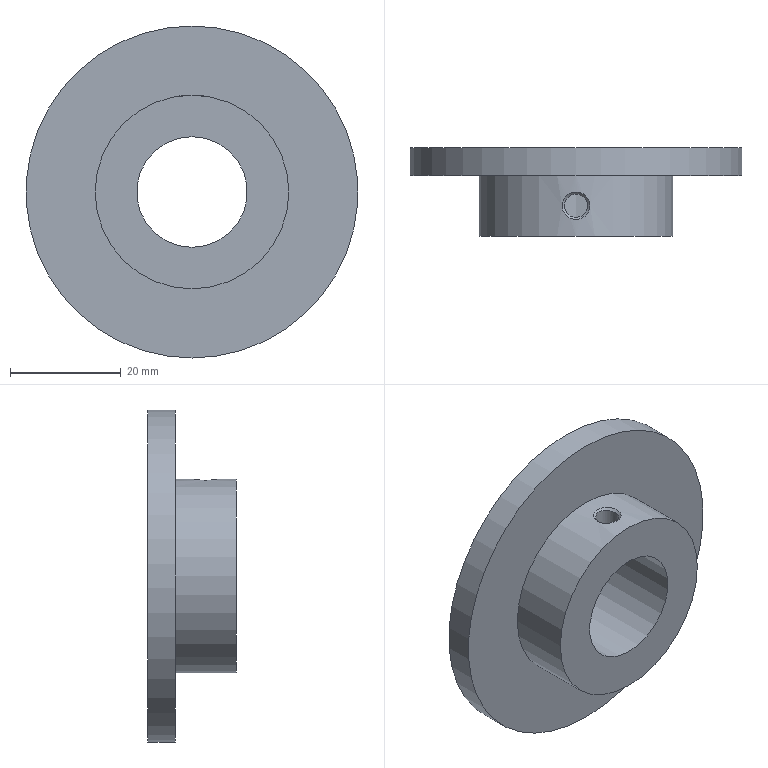Part | STEP file | 冲床-300配套压波_id698_x_t | 1 solid | 9 faces | box 60 x 16 x 60 mm | volume 19587 mm3 | cylinder 4 | plane 3 | spline 2 | commonest cylinder face diameters 4.2 x1 20 x1 35 x1 60 x1
STEP:
#1=CARTESIAN_POINT('',(1917.499,-73.887,75.321));
#2=VERTEX_POINT('',#1);
#3=CARTESIAN_POINT('',(1917.499,-73.887,75.321));
#4=CARTESIAN_POINT('',(1917.394,-74.536,75.336));
#5=CARTESIAN_POINT('',(1917.031,-75.116,75.39));
#6=CARTESIAN_POINT('',(1916.488,-75.502,75.437));
#7=CARTESIAN_POINT('',(1915.945,-75.888,75.483));
#8=CARTESIAN_POINT('',(1915.267,-76.047,75.51));
#9=CARTESIAN_POINT('',(1914.606,-75.945,75.496));
#10=CARTESIAN_POINT('',(1913.945,-75.844,75.481));
#11=CARTESIAN_POINT('',(1913.35,-75.489,75.427));
#12=CARTESIAN_POINT('',(1912.955,-74.957,75.38));
#13=CARTESIAN_POINT('',(1912.559,-74.425,75.333));
#14=CARTESIAN_POINT('',(1912.396,-73.761,75.306));
#15=CARTESIAN_POINT('',(1912.501,-73.113,75.321));
#16=CARTESIAN_POINT('',(1912.606,-72.465,75.336));
#17=CARTESIAN_POINT('',(1912.969,-71.884,75.39));
#18=CARTESIAN_POINT('',(1913.513,-71.497,75.437));
#19=CARTESIAN_POINT('',(1914.056,-71.111,75.483));
#20=CARTESIAN_POINT('',(1914.734,-70.952,75.511));
#21=CARTESIAN_POINT('',(1915.397,-71.055,75.496));
#22=CARTESIAN_POINT('',(1916.059,-71.158,75.48));
#23=CARTESIAN_POINT('',(1916.651,-71.513,75.426));
#24=CARTESIAN_POINT('',(1917.046,-72.044,75.38));
#25=CARTESIAN_POINT('',(1917.44,-72.574,75.334));
#26=CARTESIAN_POINT('',(1917.604,-73.237,75.306));
#27=CARTESIAN_POINT('',(1917.499,-73.887,75.321));
#28=B_SPLINE_CURVE_WITH_KNOTS('',3,(#3,#4,#5,#6,#7,#8,#9,#10,#11,#12,#13,#14,#15,#16,#17,#18,#19,#20,#21,#22,#23,#24,#25,#26,#27),.UNSPECIFIED.,.T.,.F.,(1,3,3,3,3,3,3,3,3,3,1),(-0.125,0.,0.125,0.25,0.375,0.5,0.625,0.75,0.875,1.,1.125),.UNSPECIFIED.);
#29=EDGE_CURVE('',#2,#2,#28,.T.);
#30=ORIENTED_EDGE('',*,*,#29,.T.);
#31=EDGE_LOOP('',(#30));
#32=FACE_BOUND('',#31,.T.);
#33=CARTESIAN_POINT('',(1915.,-68.,40.5));
#34=VERTEX_POINT('',#33);
#35=CARTESIAN_POINT('',(1915.,-68.,58.));
#36=DIRECTION('',(0.,1.,0.));
#37=DIRECTION('',(0.,0.,-1.));
#38=AXIS2_PLACEMENT_3D('',#35,#36,#37);
#39=CIRCLE('',#38,17.5);
#40=EDGE_CURVE('',#34,#34,#39,.T.);
#41=ORIENTED_EDGE('',*,*,#40,.F.);
#42=EDGE_LOOP('',(#41));
#43=FACE_BOUND('',#42,.T.);
#44=CARTESIAN_POINT('',(1915.,-79.,40.5));
#45=VERTEX_POINT('',#44);
#46=CARTESIAN_POINT('',(1915.,-79.,58.));
#47=DIRECTION('',(0.,1.,0.));
#48=DIRECTION('',(0.,0.,-1.));
#49=AXIS2_PLACEMENT_3D('',#46,#47,#48);
#50=CIRCLE('',#49,17.5);
#51=EDGE_CURVE('',#45,#45,#50,.T.);
#52=ORIENTED_EDGE('',*,*,#51,.T.);
#53=EDGE_LOOP('',(#52));
#54=FACE_BOUND('',#53,.T.);
#55=CARTESIAN_POINT('',(1915.,-68.,58.));
#56=DIRECTION('',(0.,-1.,0.));
#57=DIRECTION('',(0.,0.,-1.));
#58=AXIS2_PLACEMENT_3D('',#55,#56,#57);
#59=CYLINDRICAL_SURFACE('',#58,17.5);
#60=ADVANCED_FACE('',(#32,#43,#54),#59,.T.);
#61=CARTESIAN_POINT('',(1912.643,-72.847,67.718));
#62=VERTEX_POINT('',#61);
#63=CARTESIAN_POINT('',(1912.643,-72.847,67.718));
#64=CARTESIAN_POINT('',(1912.476,-73.503,67.678));
#65=CARTESIAN_POINT('',(1912.566,-74.199,67.705));
#66=CARTESIAN_POINT('',(1912.894,-74.785,67.776));
#67=CARTESIAN_POINT('',(1913.221,-75.37,67.846));
#68=CARTESIAN_POINT('',(1913.751,-75.79,67.941));
#69=CARTESIAN_POINT('',(1914.375,-75.963,67.98));
#70=CARTESIAN_POINT('',(1914.999,-76.136,68.02));
#71=CARTESIAN_POINT('',(1915.669,-76.042,67.994));
#72=CARTESIAN_POINT('',(1916.228,-75.701,67.924));
#73=CARTESIAN_POINT('',(1916.788,-75.36,67.855));
#74=CARTESIAN_POINT('',(1917.192,-74.804,67.758));
#75=CARTESIAN_POINT('',(1917.358,-74.151,67.718));
#76=CARTESIAN_POINT('',(1917.523,-73.498,67.678));
#77=CARTESIAN_POINT('',(1917.433,-72.801,67.705));
#78=CARTESIAN_POINT('',(1917.106,-72.216,67.776));
#79=CARTESIAN_POINT('',(1916.779,-71.63,67.846));
#80=CARTESIAN_POINT('',(1916.247,-71.209,67.942));
#81=CARTESIAN_POINT('',(1915.623,-71.036,67.981));
#82=CARTESIAN_POINT('',(1914.999,-70.864,68.02));
#83=CARTESIAN_POINT('',(1914.329,-70.959,67.993));
#84=CARTESIAN_POINT('',(1913.771,-71.299,67.924));
#85=CARTESIAN_POINT('',(1913.212,-71.64,67.855));
#86=CARTESIAN_POINT('',(1912.808,-72.196,67.758));
#87=CARTESIAN_POINT('',(1912.643,-72.847,67.718));
#88=B_SPLINE_CURVE_WITH_KNOTS('',3,(#63,#64,#65,#66,#67,#68,#69,#70,#71,#72,#73,#74,#75,#76,#77,#78,#79,#80,#81,#82,#83,#84,#85,#86,#87),.UNSPECIFIED.,.T.,.F.,(1,3,3,3,3,3,3,3,3,3,1),(-0.125,0.,0.125,0.25,0.375,0.5,0.625,0.75,0.875,1.,1.125),.UNSPECIFIED.);
#89=EDGE_CURVE('',#62,#62,#88,.T.);
#90=ORIENTED_EDGE('',*,*,#89,.T.);
#91=EDGE_LOOP('',(#90));
#92=FACE_BOUND('',#91,.T.);
#93=CARTESIAN_POINT('',(1915.,-79.,48.));
#94=VERTEX_POINT('',#93);
#95=CARTESIAN_POINT('',(1915.,-79.,58.));
#96=DIRECTION('',(0.,1.,0.));
#97=DIRECTION('',(0.,0.,-1.));
#98=AXIS2_PLACEMENT_3D('',#95,#96,#97);
#99=CIRCLE('',#98,10.);
#100=EDGE_CURVE('',#94,#94,#99,.T.);
#101=ORIENTED_EDGE('',*,*,#100,.F.);
#102=EDGE_LOOP('',(#101));
#103=FACE_BOUND('',#102,.T.);
#104=CARTESIAN_POINT('',(1915.,-63.,68.));
#105=VERTEX_POINT('',#104);
#106=CARTESIAN_POINT('',(1915.,-63.,58.));
#107=DIRECTION('',(0.,-1.,0.));
#108=DIRECTION('',(0.,0.,1.));
#109=AXIS2_PLACEMENT_3D('',#106,#107,#108);
#110=CIRCLE('',#109,10.);
#111=EDGE_CURVE('',#105,#105,#110,.T.);
#112=ORIENTED_EDGE('',*,*,#111,.F.);
#113=EDGE_LOOP('',(#112));
#114=FACE_BOUND('',#113,.T.);
#115=CARTESIAN_POINT('',(1915.,-68.,58.));
#116=DIRECTION('',(0.,-1.,0.));
#117=DIRECTION('',(0.,0.,-1.));
#118=AXIS2_PLACEMENT_3D('',#115,#116,#117);
#119=CYLINDRICAL_SURFACE('',#118,10.);
#120=ADVANCED_FACE('',(#92,#103,#114),#119,.F.);
#121=ORIENTED_EDGE('',*,*,#51,.F.);
#122=EDGE_LOOP('',(#121));
#123=FACE_BOUND('',#122,.T.);
#124=ORIENTED_EDGE('',*,*,#100,.T.);
#125=EDGE_LOOP('',(#124));
#126=FACE_BOUND('',#125,.T.);
#127=CARTESIAN_POINT('',(1915.,-79.,58.));
#128=DIRECTION('',(0.,-1.,0.));
#129=DIRECTION('',(0.,0.,-1.));
#130=AXIS2_PLACEMENT_3D('',#127,#128,#129);
#131=PLANE('',#130);
#132=ADVANCED_FACE('',(#123,#126),#131,.T.);
#133=ORIENTED_EDGE('',*,*,#111,.T.);
#134=EDGE_LOOP('',(#133));
#135=FACE_BOUND('',#134,.T.);
#136=CARTESIAN_POINT('',(1915.,-63.,88.));
#137=VERTEX_POINT('',#136);
#138=CARTESIAN_POINT('',(1915.,-63.,58.));
#139=DIRECTION('',(0.,1.,0.));
#140=DIRECTION('',(0.,0.,1.));
#141=AXIS2_PLACEMENT_3D('',#138,#139,#140);
#142=CIRCLE('',#141,30.);
#143=EDGE_CURVE('',#137,#137,#142,.T.);
#144=ORIENTED_EDGE('',*,*,#143,.T.);
#145=EDGE_LOOP('',(#144));
#146=FACE_BOUND('',#145,.T.);
#147=CARTESIAN_POINT('',(1915.,-63.,58.));
#148=DIRECTION('',(0.,1.,0.));
#149=DIRECTION('',(0.,0.,1.));
#150=AXIS2_PLACEMENT_3D('',#147,#148,#149);
#151=PLANE('',#150);
#152=ADVANCED_FACE('',(#135,#146),#151,.T.);
#153=ORIENTED_EDGE('',*,*,#40,.T.);
#154=EDGE_LOOP('',(#153));
#155=FACE_BOUND('',#154,.T.);
#156=CARTESIAN_POINT('',(1915.,-68.,28.));
#157=VERTEX_POINT('',#156);
#158=CARTESIAN_POINT('',(1915.,-68.,58.));
#159=DIRECTION('',(0.,-1.,0.));
#160=DIRECTION('',(0.,0.,-1.));
#161=AXIS2_PLACEMENT_3D('',#158,#159,#160);
#162=CIRCLE('',#161,30.);
#163=EDGE_CURVE('',#157,#157,#162,.T.);
#164=ORIENTED_EDGE('',*,*,#163,.T.);
#165=EDGE_LOOP('',(#164));
#166=FACE_BOUND('',#165,.T.);
#167=CARTESIAN_POINT('',(1915.,-68.,58.));
#168=DIRECTION('',(0.,-1.,0.));
#169=DIRECTION('',(0.,0.,-1.));
#170=AXIS2_PLACEMENT_3D('',#167,#168,#169);
#171=PLANE('',#170);
#172=ADVANCED_FACE('',(#155,#166),#171,.T.);
#173=ORIENTED_EDGE('',*,*,#143,.F.);
#174=EDGE_LOOP('',(#173));
#175=FACE_BOUND('',#174,.T.);
#176=ORIENTED_EDGE('',*,*,#163,.F.);
#177=EDGE_LOOP('',(#176));
#178=FACE_BOUND('',#177,.T.);
#179=CARTESIAN_POINT('',(1915.,80.,58.));
#180=DIRECTION('',(0.,-1.,0.));
#181=DIRECTION('',(0.,0.,-1.));
#182=AXIS2_PLACEMENT_3D('',#179,#180,#181);
#183=CYLINDRICAL_SURFACE('',#182,30.);
#184=ADVANCED_FACE('',(#175,#178),#183,.T.);
#185=CARTESIAN_POINT('',(1917.074,-73.828,74.949));
#186=VERTEX_POINT('',#185);
#187=CARTESIAN_POINT('',(1917.074,-73.828,74.949));
#188=CARTESIAN_POINT('',(1917.117,-73.559,74.942));
#189=CARTESIAN_POINT('',(1917.096,-73.233,74.945));
#190=CARTESIAN_POINT('',(1917.042,-73.008,74.954));
#191=CARTESIAN_POINT('',(1917.014,-72.895,74.959));
#192=CARTESIAN_POINT('',(1916.975,-72.774,74.966));
#193=CARTESIAN_POINT('',(1916.92,-72.649,74.974));
#194=CARTESIAN_POINT('',(1916.892,-72.586,74.979));
#195=CARTESIAN_POINT('',(1916.86,-72.522,74.984));
#196=CARTESIAN_POINT('',(1916.823,-72.458,74.989));
#197=CARTESIAN_POINT('',(1916.786,-72.393,74.994));
#198=CARTESIAN_POINT('',(1916.715,-72.288,75.005));
#199=CARTESIAN_POINT('',(1916.698,-72.265,75.007));
#200=CARTESIAN_POINT('',(1916.664,-72.217,75.012));
#201=CARTESIAN_POINT('',(1916.549,-72.072,75.027));
#202=CARTESIAN_POINT('',(1916.426,-71.958,75.042));
#203=CARTESIAN_POINT('',(1916.302,-71.844,75.056));
#204=CARTESIAN_POINT('',(1916.227,-71.789,75.064));
#205=CARTESIAN_POINT('',(1916.097,-71.71,75.075));
#206=CARTESIAN_POINT('',(1915.837,-71.55,75.099));
#207=CARTESIAN_POINT('',(1915.598,-71.469,75.113));
#208=CARTESIAN_POINT('',(1915.329,-71.426,75.12));
#209=CARTESIAN_POINT('',(1915.061,-71.383,75.127));
#210=CARTESIAN_POINT('',(1914.736,-71.404,75.124));
#211=CARTESIAN_POINT('',(1914.51,-71.458,75.115));
#212=CARTESIAN_POINT('',(1914.396,-71.485,75.11));
#213=CARTESIAN_POINT('',(1914.275,-71.524,75.103));
#214=CARTESIAN_POINT('',(1914.149,-71.58,75.095));
#215=CARTESIAN_POINT('',(1914.087,-71.608,75.09));
#216=CARTESIAN_POINT('',(1914.023,-71.64,75.086));
#217=CARTESIAN_POINT('',(1913.958,-71.677,75.08));
#218=CARTESIAN_POINT('',(1913.894,-71.713,75.075));
#219=CARTESIAN_POINT('',(1913.792,-71.782,75.065));
#220=CARTESIAN_POINT('',(1913.765,-71.801,75.062));
#221=CARTESIAN_POINT('',(1913.713,-71.84,75.057));
#222=CARTESIAN_POINT('',(1913.574,-71.949,75.042));
#223=CARTESIAN_POINT('',(1913.458,-72.074,75.028));
#224=CARTESIAN_POINT('',(1913.343,-72.199,75.013));
#225=CARTESIAN_POINT('',(1913.29,-72.272,75.005));
#226=CARTESIAN_POINT('',(1913.21,-72.403,74.994));
#227=CARTESIAN_POINT('',(1913.049,-72.664,74.97));
#228=CARTESIAN_POINT('',(1912.969,-72.898,74.956));
#229=CARTESIAN_POINT('',(1912.926,-73.172,74.949));
#230=CARTESIAN_POINT('',(1912.882,-73.446,74.941));
#231=CARTESIAN_POINT('',(1912.892,-73.712,74.943));
#232=CARTESIAN_POINT('',(1912.956,-73.984,74.954));
#233=CARTESIAN_POINT('',(1913.021,-74.255,74.965));
#234=CARTESIAN_POINT('',(1913.104,-74.453,74.98));
#235=CARTESIAN_POINT('',(1913.277,-74.7,75.004));
#236=CARTESIAN_POINT('',(1913.449,-74.948,75.028));
#237=CARTESIAN_POINT('',(1913.764,-75.212,75.063));
#238=CARTESIAN_POINT('',(1913.957,-75.322,75.08));
#239=CARTESIAN_POINT('',(1914.149,-75.432,75.097));
#240=CARTESIAN_POINT('',(1914.421,-75.536,75.113));
#241=CARTESIAN_POINT('',(1914.682,-75.576,75.12));
#242=CARTESIAN_POINT('',(1914.942,-75.616,75.127));
#243=CARTESIAN_POINT('',(1915.216,-75.608,75.125));
#244=CARTESIAN_POINT('',(1915.489,-75.542,75.115));
#245=CARTESIAN_POINT('',(1915.761,-75.477,75.104));
#246=CARTESIAN_POINT('',(1915.97,-75.389,75.089));
#247=CARTESIAN_POINT('',(1916.224,-75.206,75.063));
#248=CARTESIAN_POINT('',(1916.288,-75.16,75.057));
#249=CARTESIAN_POINT('',(1916.318,-75.136,75.054));
#250=CARTESIAN_POINT('',(1916.365,-75.096,75.049));
#251=CARTESIAN_POINT('',(1916.411,-75.056,75.043));
#252=CARTESIAN_POINT('',(1916.488,-74.984,75.034));
#253=CARTESIAN_POINT('',(1916.546,-74.921,75.027));
#254=CARTESIAN_POINT('',(1916.661,-74.796,75.013));
#255=CARTESIAN_POINT('',(1916.74,-74.681,75.001));
#256=CARTESIAN_POINT('',(1916.796,-74.589,74.993));
#257=CARTESIAN_POINT('',(1916.851,-74.497,74.985));
#258=CARTESIAN_POINT('',(1916.931,-74.338,74.973));
#259=CARTESIAN_POINT('',(1916.977,-74.207,74.965));
#260=CARTESIAN_POINT('',(1917.024,-74.077,74.958));
#261=CARTESIAN_POINT('',(1917.055,-73.95,74.952));
#262=CARTESIAN_POINT('',(1917.074,-73.828,74.949));
#263=B_SPLINE_CURVE_WITH_KNOTS('',3,(#187,#188,#189,#190,#191,#192,#193,#194,#195,#196,#197,#198,#199,#200,#201,#202,#203,#204,#205,#206,#207,#208,#209,#210,#211,#212,#213,#214,#215,#216,#217,#218,#219,#220,#221,#222,#223,#224,#225,#226,#227,#228,#229,#230,#231,#232,#233,#234,#235,#236,#237,#238,#239,#240,#241,#242,#243,#244,#245,#246,#247,#248,#249,#250,#251,#252,#253,#254,#255,#256,#257,#258,#259,#260,#261,#262),.UNSPECIFIED.,.T.,.F.,(1,3,3,3,3,3,3,3,3,3,3,3,3,3,3,3,3,3,3,3,3,3,3,3,3,3,3,1),(-0.04,0.,0.04,0.08,0.12,0.16,0.2,0.24,0.28,0.32,0.36,0.4,0.44,0.48,0.52,0.56,0.6,0.64,0.68,0.72,0.76,0.8,0.84,0.88,0.92,0.96,1.,1.04),.UNSPECIFIED.);
#264=EDGE_CURVE('',#186,#186,#263,.T.);
#265=ORIENTED_EDGE('',*,*,#264,.T.);
#266=EDGE_LOOP('',(#265));
#267=FACE_BOUND('',#266,.T.);
#268=CARTESIAN_POINT('',(1912.97,-72.962,68.154));
#269=VERTEX_POINT('',#268);
#270=CARTESIAN_POINT('',(1912.97,-72.962,68.154));
#271=CARTESIAN_POINT('',(1913.028,-72.743,68.171));
#272=CARTESIAN_POINT('',(1913.164,-72.444,68.21));
#273=CARTESIAN_POINT('',(1913.33,-72.227,68.25));
#274=CARTESIAN_POINT('',(1913.495,-72.01,68.289));
#275=CARTESIAN_POINT('',(1913.681,-71.839,68.33));
#276=CARTESIAN_POINT('',(1913.941,-71.686,68.369));
#277=CARTESIAN_POINT('',(1914.202,-71.534,68.408));
#278=CARTESIAN_POINT('',(1914.448,-71.456,68.432));
#279=CARTESIAN_POINT('',(1914.716,-71.419,68.442));
#280=CARTESIAN_POINT('',(1914.985,-71.383,68.453));
#281=CARTESIAN_POINT('',(1915.314,-71.411,68.445));
#282=CARTESIAN_POINT('',(1915.536,-71.47,68.428));
#283=CARTESIAN_POINT('',(1915.648,-71.499,68.419));
#284=CARTESIAN_POINT('',(1915.767,-71.54,68.407));
#285=CARTESIAN_POINT('',(1915.892,-71.599,68.392));
#286=CARTESIAN_POINT('',(1915.954,-71.628,68.384));
#287=CARTESIAN_POINT('',(1916.017,-71.661,68.375));
#288=CARTESIAN_POINT('',(1916.081,-71.7,68.365));
#289=CARTESIAN_POINT('',(1916.113,-71.719,68.36));
#290=CARTESIAN_POINT('',(1916.145,-71.739,68.355));
#291=CARTESIAN_POINT('',(1916.177,-71.761,68.35));
#292=CARTESIAN_POINT('',(1916.209,-71.782,68.345));
#293=CARTESIAN_POINT('',(1916.265,-71.824,68.335));
#294=CARTESIAN_POINT('',(1916.272,-71.829,68.333));
#295=CARTESIAN_POINT('',(1916.287,-71.841,68.331));
#296=CARTESIAN_POINT('',(1916.322,-71.867,68.324));
#297=CARTESIAN_POINT('',(1916.374,-71.912,68.314));
#298=CARTESIAN_POINT('',(1916.425,-71.956,68.304));
#299=CARTESIAN_POINT('',(1916.517,-72.046,68.285));
#300=CARTESIAN_POINT('',(1916.573,-72.108,68.272));
#301=CARTESIAN_POINT('',(1916.683,-72.233,68.248));
#302=CARTESIAN_POINT('',(1916.737,-72.31,68.234));
#303=CARTESIAN_POINT('',(1916.814,-72.441,68.214));
#304=CARTESIAN_POINT('',(1916.967,-72.704,68.174));
#305=CARTESIAN_POINT('',(1917.044,-72.948,68.149));
#306=CARTESIAN_POINT('',(1917.081,-73.217,68.138));
#307=CARTESIAN_POINT('',(1917.117,-73.485,68.127));
#308=CARTESIAN_POINT('',(1917.088,-73.816,68.136));
#309=CARTESIAN_POINT('',(1917.03,-74.036,68.153));
#310=CARTESIAN_POINT('',(1916.972,-74.256,68.171));
#311=CARTESIAN_POINT('',(1916.836,-74.555,68.21));
#312=CARTESIAN_POINT('',(1916.67,-74.773,68.25));
#313=CARTESIAN_POINT('',(1916.504,-74.991,68.29));
#314=CARTESIAN_POINT('',(1916.319,-75.162,68.33));
#315=CARTESIAN_POINT('',(1916.058,-75.314,68.369));
#316=CARTESIAN_POINT('',(1915.796,-75.467,68.408));
#317=CARTESIAN_POINT('',(1915.551,-75.545,68.432));
#318=CARTESIAN_POINT('',(1915.282,-75.581,68.442));
#319=CARTESIAN_POINT('',(1915.012,-75.617,68.453));
#320=CARTESIAN_POINT('',(1914.685,-75.589,68.445));
#321=CARTESIAN_POINT('',(1914.462,-75.53,68.428));
#322=CARTESIAN_POINT('',(1914.35,-75.5,68.419));
#323=CARTESIAN_POINT('',(1914.231,-75.459,68.407));
#324=CARTESIAN_POINT('',(1914.106,-75.4,68.391));
#325=CARTESIAN_POINT('',(1914.044,-75.371,68.383));
#326=CARTESIAN_POINT('',(1913.981,-75.338,68.375));
#327=CARTESIAN_POINT('',(1913.918,-75.3,68.365));
#328=CARTESIAN_POINT('',(1913.886,-75.281,68.36));
#329=CARTESIAN_POINT('',(1913.854,-75.26,68.355));
#330=CARTESIAN_POINT('',(1913.822,-75.239,68.35));
#331=CARTESIAN_POINT('',(1913.791,-75.217,68.345));
#332=CARTESIAN_POINT('',(1913.734,-75.176,68.335));
#333=CARTESIAN_POINT('',(1913.727,-75.17,68.333));
#334=CARTESIAN_POINT('',(1913.713,-75.159,68.331));
#335=CARTESIAN_POINT('',(1913.678,-75.133,68.324));
#336=CARTESIAN_POINT('',(1913.626,-75.088,68.314));
#337=CARTESIAN_POINT('',(1913.574,-75.043,68.304));
#338=CARTESIAN_POINT('',(1913.481,-74.952,68.284));
#339=CARTESIAN_POINT('',(1913.426,-74.89,68.272));
#340=CARTESIAN_POINT('',(1913.317,-74.767,68.247));
#341=CARTESIAN_POINT('',(1913.262,-74.688,68.233));
#342=CARTESIAN_POINT('',(1913.186,-74.559,68.214));
#343=CARTESIAN_POINT('',(1912.884,-74.04,68.135));
#344=CARTESIAN_POINT('',(1912.826,-73.507,68.111));
#345=CARTESIAN_POINT('',(1912.97,-72.962,68.154));
#346=B_SPLINE_CURVE_WITH_KNOTS('',3,(#270,#271,#272,#273,#274,#275,#276,#277,#278,#279,#280,#281,#282,#283,#284,#285,#286,#287,#288,#289,#290,#291,#292,#293,#294,#295,#296,#297,#298,#299,#300,#301,#302,#303,#304,#305,#306,#307,#308,#309,#310,#311,#312,#313,#314,#315,#316,#317,#318,#319,#320,#321,#322,#323,#324,#325,#326,#327,#328,#329,#330,#331,#332,#333,#334,#335,#336,#337,#338,#339,#340,#341,#342,#343,#344,#345),.UNSPECIFIED.,.T.,.F.,(1,3,3,3,3,3,3,3,3,3,3,3,3,3,3,3,3,3,3,3,3,3,3,3,3,3,3,1),(-0.04,0.,0.04,0.08,0.12,0.16,0.2,0.24,0.28,0.32,0.36,0.4,0.44,0.48,0.52,0.56,0.6,0.64,0.68,0.72,0.76,0.8,0.84,0.88,0.92,0.96,1.,1.04),.UNSPECIFIED.);
#347=EDGE_CURVE('',#269,#269,#346,.T.);
#348=ORIENTED_EDGE('',*,*,#347,.T.);
#349=EDGE_LOOP('',(#348));
#350=FACE_BOUND('',#349,.T.);
#351=CARTESIAN_POINT('',(1915.,-73.5,93.));
#352=DIRECTION('',(0.,0.,-1.));
#353=DIRECTION('',(-1.,0.,0.));
#354=AXIS2_PLACEMENT_3D('',#351,#352,#353);
#355=CYLINDRICAL_SURFACE('',#354,2.1);
#356=ADVANCED_FACE('',(#267,#350),#355,.F.);
#357=ORIENTED_EDGE('',*,*,#347,.F.);
#358=EDGE_LOOP('',(#357));
#359=FACE_BOUND('',#358,.T.);
#360=ORIENTED_EDGE('',*,*,#89,.F.);
#361=EDGE_LOOP('',(#360));
#362=FACE_BOUND('',#361,.T.);
#363=CARTESIAN_POINT('',(1912.684,-72.685,67.728));
#364=CARTESIAN_POINT('',(1912.601,-73.009,67.708));
#365=CARTESIAN_POINT('',(1912.576,-73.177,67.702));
#366=CARTESIAN_POINT('',(1912.556,-73.508,67.697));
#367=CARTESIAN_POINT('',(1912.562,-73.676,67.698));
#368=CARTESIAN_POINT('',(1912.605,-74.011,67.709));
#369=CARTESIAN_POINT('',(1912.642,-74.173,67.718));
#370=CARTESIAN_POINT('',(1912.746,-74.487,67.743));
#371=CARTESIAN_POINT('',(1912.813,-74.641,67.758));
#372=CARTESIAN_POINT('',(1912.974,-74.928,67.793));
#373=CARTESIAN_POINT('',(1913.067,-75.062,67.812));
#374=CARTESIAN_POINT('',(1913.278,-75.312,67.851));
#375=CARTESIAN_POINT('',(1913.396,-75.427,67.871));
#376=CARTESIAN_POINT('',(1913.773,-75.727,67.928));
#377=CARTESIAN_POINT('',(1914.068,-75.878,67.961));
#378=CARTESIAN_POINT('',(1914.528,-76.005,67.99));
#379=CARTESIAN_POINT('',(1914.688,-76.033,67.996));
#380=CARTESIAN_POINT('',(1915.01,-76.054,68.001));
#381=CARTESIAN_POINT('',(1915.169,-76.047,68.));
#382=CARTESIAN_POINT('',(1915.485,-76.003,67.989));
#383=CARTESIAN_POINT('',(1915.644,-75.963,67.98));
#384=CARTESIAN_POINT('',(1915.945,-75.855,67.956));
#385=CARTESIAN_POINT('',(1916.09,-75.786,67.941));
#386=CARTESIAN_POINT('',(1916.505,-75.533,67.89));
#387=CARTESIAN_POINT('',(1916.746,-75.31,67.848));
#388=CARTESIAN_POINT('',(1917.037,-74.912,67.791));
#389=CARTESIAN_POINT('',(1917.12,-74.77,67.773));
#390=CARTESIAN_POINT('',(1917.261,-74.47,67.741));
#391=CARTESIAN_POINT('',(1917.317,-74.311,67.728));
#392=CARTESIAN_POINT('',(1917.439,-73.83,67.698));
#393=CARTESIAN_POINT('',(1917.46,-73.486,67.693));
#394=CARTESIAN_POINT('',(1917.395,-72.991,67.709));
#395=CARTESIAN_POINT('',(1917.357,-72.826,67.718));
#396=CARTESIAN_POINT('',(1917.253,-72.51,67.743));
#397=CARTESIAN_POINT('',(1917.187,-72.36,67.758));
#398=CARTESIAN_POINT('',(1917.026,-72.072,67.793));
#399=CARTESIAN_POINT('',(1916.931,-71.935,67.812));
#400=CARTESIAN_POINT('',(1916.721,-71.688,67.851));
#401=CARTESIAN_POINT('',(1916.605,-71.574,67.871));
#402=CARTESIAN_POINT('',(1916.35,-71.371,67.909));
#403=CARTESIAN_POINT('',(1916.214,-71.284,67.927));
#404=CARTESIAN_POINT('',(1915.93,-71.138,67.958));
#405=CARTESIAN_POINT('',(1915.778,-71.079,67.971));
#406=CARTESIAN_POINT('',(1915.468,-70.994,67.99));
#407=CARTESIAN_POINT('',(1915.31,-70.967,67.996));
#408=CARTESIAN_POINT('',(1914.992,-70.946,68.001));
#409=CARTESIAN_POINT('',(1914.828,-70.953,68.));
#410=CARTESIAN_POINT('',(1914.512,-70.998,67.989));
#411=CARTESIAN_POINT('',(1914.358,-71.036,67.981));
#412=CARTESIAN_POINT('',(1914.053,-71.146,67.956));
#413=CARTESIAN_POINT('',(1913.907,-71.216,67.941));
#414=CARTESIAN_POINT('',(1913.634,-71.383,67.907));
#415=CARTESIAN_POINT('',(1913.504,-71.481,67.888));
#416=CARTESIAN_POINT('',(1913.264,-71.703,67.849));
#417=CARTESIAN_POINT('',(1913.156,-71.824,67.829));
#418=CARTESIAN_POINT('',(1912.964,-72.087,67.791));
#419=CARTESIAN_POINT('',(1912.879,-72.231,67.773));
#420=CARTESIAN_POINT('',(1912.739,-72.53,67.741));
#421=CARTESIAN_POINT('',(1912.684,-72.685,67.728));
#422=CARTESIAN_POINT('',(1912.601,-73.009,67.708));
#423=CARTESIAN_POINT('',(1913.006,-72.828,68.164));
#424=CARTESIAN_POINT('',(1912.935,-73.095,68.143));
#425=CARTESIAN_POINT('',(1912.912,-73.233,68.136));
#426=CARTESIAN_POINT('',(1912.896,-73.507,68.131));
#427=CARTESIAN_POINT('',(1912.9,-73.645,68.133));
#428=CARTESIAN_POINT('',(1912.938,-73.921,68.144));
#429=CARTESIAN_POINT('',(1912.97,-74.054,68.154));
#430=CARTESIAN_POINT('',(1913.059,-74.313,68.179));
#431=CARTESIAN_POINT('',(1913.117,-74.44,68.196));
#432=CARTESIAN_POINT('',(1913.256,-74.677,68.232));
#433=CARTESIAN_POINT('',(1913.335,-74.788,68.252));
#434=CARTESIAN_POINT('',(1913.517,-74.993,68.293));
#435=CARTESIAN_POINT('',(1913.619,-75.088,68.314));
#436=CARTESIAN_POINT('',(1913.944,-75.335,68.373));
#437=CARTESIAN_POINT('',(1914.198,-75.46,68.408));
#438=CARTESIAN_POINT('',(1914.594,-75.565,68.438));
#439=CARTESIAN_POINT('',(1914.732,-75.587,68.444));
#440=CARTESIAN_POINT('',(1915.008,-75.605,68.449));
#441=CARTESIAN_POINT('',(1915.145,-75.599,68.448));
#442=CARTESIAN_POINT('',(1915.418,-75.563,68.437));
#443=CARTESIAN_POINT('',(1915.555,-75.53,68.428));
#444=CARTESIAN_POINT('',(1915.814,-75.441,68.402));
#445=CARTESIAN_POINT('',(1915.938,-75.384,68.387));
#446=CARTESIAN_POINT('',(1916.296,-75.175,68.333));
#447=CARTESIAN_POINT('',(1916.503,-74.992,68.29));
#448=CARTESIAN_POINT('',(1916.754,-74.663,68.23));
#449=CARTESIAN_POINT('',(1916.826,-74.547,68.211));
#450=CARTESIAN_POINT('',(1916.947,-74.3,68.178));
#451=CARTESIAN_POINT('',(1916.995,-74.169,68.164));
#452=CARTESIAN_POINT('',(1917.1,-73.772,68.133));
#453=CARTESIAN_POINT('',(1917.118,-73.488,68.127));
#454=CARTESIAN_POINT('',(1917.062,-73.081,68.144));
#455=CARTESIAN_POINT('',(1917.03,-72.944,68.154));
#456=CARTESIAN_POINT('',(1916.94,-72.684,68.18));
#457=CARTESIAN_POINT('',(1916.883,-72.56,68.196));
#458=CARTESIAN_POINT('',(1916.744,-72.323,68.232));
#459=CARTESIAN_POINT('',(1916.663,-72.21,68.252));
#460=CARTESIAN_POINT('',(1916.482,-72.006,68.293));
#461=CARTESIAN_POINT('',(1916.382,-71.913,68.313));
#462=CARTESIAN_POINT('',(1916.162,-71.746,68.353));
#463=CARTESIAN_POINT('',(1916.045,-71.674,68.372));
#464=CARTESIAN_POINT('',(1915.8,-71.554,68.404));
#465=CARTESIAN_POINT('',(1915.67,-71.505,68.418));
#466=CARTESIAN_POINT('',(1915.403,-71.434,68.438));
#467=CARTESIAN_POINT('',(1915.267,-71.413,68.444));
#468=CARTESIAN_POINT('',(1914.993,-71.395,68.449));
#469=CARTESIAN_POINT('',(1914.852,-71.401,68.448));
#470=CARTESIAN_POINT('',(1914.58,-71.438,68.437));
#471=CARTESIAN_POINT('',(1914.447,-71.469,68.428));
#472=CARTESIAN_POINT('',(1914.185,-71.56,68.402));
#473=CARTESIAN_POINT('',(1914.059,-71.618,68.386));
#474=CARTESIAN_POINT('',(1913.823,-71.755,68.351));
#475=CARTESIAN_POINT('',(1913.711,-71.836,68.331));
#476=CARTESIAN_POINT('',(1913.505,-72.019,68.29));
#477=CARTESIAN_POINT('',(1913.412,-72.119,68.269));
#478=CARTESIAN_POINT('',(1913.247,-72.336,68.23));
#479=CARTESIAN_POINT('',(1913.174,-72.454,68.211));
#480=CARTESIAN_POINT('',(1913.053,-72.7,68.178));
#481=CARTESIAN_POINT('',(1913.006,-72.828,68.164));
#482=CARTESIAN_POINT('',(1912.935,-73.095,68.143));
#483=B_SPLINE_SURFACE_WITH_KNOTS('',1,3,((#363,#364,#365,#366,#367,#368,#369,#370,#371,#372,#373,#374,#375,#376,#377,#378,#379,#380,#381,#382,#383,#384,#385,#386,#387,#388,#389,#390,#391,#392,#393,#394,#395,#396,#397,#398,#399,#400,#401,#402,#403,#404,#405,#406,#407,#408,#409,#410,#411,#412,#413,#414,#415,#416,#417,#418,#419,#420,#421,#422),(#423,#424,#425,#426,#427,#428,#429,#430,#431,#432,#433,#434,#435,#436,#437,#438,#439,#440,#441,#442,#443,#444,#445,#446,#447,#448,#449,#450,#451,#452,#453,#454,#455,#456,#457,#458,#459,#460,#461,#462,#463,#464,#465,#466,#467,#468,#469,#470,#471,#472,#473,#474,#475,#476,#477,#478,#479,#480,#481,#482)),.UNSPECIFIED.,.F.,.T.,.F.,(2,2),(2,2,2,2,2,2,2,2,2,2,2,2,2,2,2,2,2,2,2,2,2,2,2,2,2,2,2,2,2,2,2,2),(0.,1.),(-0.03125,0.,0.03125,0.0625,0.09375,0.125,0.1562,0.1875,0.25,0.2812,0.3125,0.3438,0.375,0.4375,0.4688,0.5,0.5625,0.5937,0.625,0.6562,0.6875,0.7187,0.75,0.7812,0.8125,0.8437,0.875,0.9062,0.9375,0.9687,1.,1.031),.UNSPECIFIED.);
#484=ADVANCED_FACE('',(#359,#362),#483,.T.);
#485=ORIENTED_EDGE('',*,*,#29,.F.);
#486=EDGE_LOOP('',(#485));
#487=FACE_BOUND('',#486,.T.);
#488=ORIENTED_EDGE('',*,*,#264,.F.);
#489=EDGE_LOOP('',(#488));
#490=FACE_BOUND('',#489,.T.);
#491=CARTESIAN_POINT('',(1917.053,-73.964,74.952));
#492=CARTESIAN_POINT('',(1917.096,-73.69,74.945));
#493=CARTESIAN_POINT('',(1917.104,-73.553,74.944));
#494=CARTESIAN_POINT('',(1917.093,-73.279,74.946));
#495=CARTESIAN_POINT('',(1917.074,-73.141,74.949));
#496=CARTESIAN_POINT('',(1917.009,-72.873,74.96));
#497=CARTESIAN_POINT('',(1916.964,-72.744,74.967));
#498=CARTESIAN_POINT('',(1916.849,-72.495,74.985));
#499=CARTESIAN_POINT('',(1916.778,-72.374,74.996));
#500=CARTESIAN_POINT('',(1916.617,-72.153,75.018));
#501=CARTESIAN_POINT('',(1916.526,-72.051,75.03));
#502=CARTESIAN_POINT('',(1916.323,-71.863,75.054));
#503=CARTESIAN_POINT('',(1916.213,-71.78,75.065));
#504=CARTESIAN_POINT('',(1915.98,-71.638,75.086));
#505=CARTESIAN_POINT('',(1915.856,-71.577,75.095));
#506=CARTESIAN_POINT('',(1915.596,-71.482,75.111));
#507=CARTESIAN_POINT('',(1915.463,-71.447,75.116));
#508=CARTESIAN_POINT('',(1915.193,-71.404,75.124));
#509=CARTESIAN_POINT('',(1915.053,-71.396,75.125));
#510=CARTESIAN_POINT('',(1914.778,-71.407,75.123));
#511=CARTESIAN_POINT('',(1914.643,-71.426,75.12));
#512=CARTESIAN_POINT('',(1914.374,-71.491,75.109));
#513=CARTESIAN_POINT('',(1914.243,-71.536,75.102));
#514=CARTESIAN_POINT('',(1913.995,-71.651,75.084));
#515=CARTESIAN_POINT('',(1913.876,-71.72,75.074));
#516=CARTESIAN_POINT('',(1913.652,-71.884,75.051));
#517=CARTESIAN_POINT('',(1913.55,-71.975,75.039));
#518=CARTESIAN_POINT('',(1913.365,-72.175,75.016));
#519=CARTESIAN_POINT('',(1913.281,-72.286,75.004));
#520=CARTESIAN_POINT('',(1913.137,-72.521,74.983));
#521=CARTESIAN_POINT('',(1913.078,-72.644,74.974));
#522=CARTESIAN_POINT('',(1912.982,-72.901,74.958));
#523=CARTESIAN_POINT('',(1912.947,-73.037,74.952));
#524=CARTESIAN_POINT('',(1912.904,-73.309,74.945));
#525=CARTESIAN_POINT('',(1912.896,-73.449,74.944));
#526=CARTESIAN_POINT('',(1912.907,-73.724,74.946));
#527=CARTESIAN_POINT('',(1912.926,-73.859,74.949));
#528=CARTESIAN_POINT('',(1912.991,-74.127,74.96));
#529=CARTESIAN_POINT('',(1913.037,-74.259,74.967));
#530=CARTESIAN_POINT('',(1913.152,-74.507,74.985));
#531=CARTESIAN_POINT('',(1913.221,-74.625,74.996));
#532=CARTESIAN_POINT('',(1913.385,-74.849,75.018));
#533=CARTESIAN_POINT('',(1913.476,-74.951,75.03));
#534=CARTESIAN_POINT('',(1913.676,-75.136,75.054));
#535=CARTESIAN_POINT('',(1913.787,-75.22,75.065));
#536=CARTESIAN_POINT('',(1914.023,-75.364,75.086));
#537=CARTESIAN_POINT('',(1914.146,-75.423,75.095));
#538=CARTESIAN_POINT('',(1914.403,-75.518,75.111));
#539=CARTESIAN_POINT('',(1914.539,-75.553,75.116));
#540=CARTESIAN_POINT('',(1914.809,-75.596,75.124));
#541=CARTESIAN_POINT('',(1914.946,-75.604,75.125));
#542=CARTESIAN_POINT('',(1915.223,-75.593,75.123));
#543=CARTESIAN_POINT('',(1915.36,-75.573,75.12));
#544=CARTESIAN_POINT('',(1915.626,-75.509,75.109));
#545=CARTESIAN_POINT('',(1915.757,-75.464,75.102));
#546=CARTESIAN_POINT('',(1916.008,-75.348,75.084));
#547=CARTESIAN_POINT('',(1916.126,-75.278,75.073));
#548=CARTESIAN_POINT('',(1916.346,-75.117,75.051));
#549=CARTESIAN_POINT('',(1916.451,-75.024,75.039));
#550=CARTESIAN_POINT('',(1916.637,-74.823,75.016));
#551=CARTESIAN_POINT('',(1916.719,-74.714,75.004));
#552=CARTESIAN_POINT('',(1916.863,-74.479,74.983));
#553=CARTESIAN_POINT('',(1916.924,-74.354,74.974));
#554=CARTESIAN_POINT('',(1917.018,-74.097,74.958));
#555=CARTESIAN_POINT('',(1917.053,-73.964,74.952));
#556=CARTESIAN_POINT('',(1917.096,-73.69,74.945));
#557=CARTESIAN_POINT('',(1917.473,-74.047,75.324));
#558=CARTESIAN_POINT('',(1917.525,-73.724,75.317));
#559=CARTESIAN_POINT('',(1917.534,-73.562,75.315));
#560=CARTESIAN_POINT('',(1917.521,-73.24,75.317));
#561=CARTESIAN_POINT('',(1917.498,-73.077,75.321));
#562=CARTESIAN_POINT('',(1917.42,-72.761,75.332));
#563=CARTESIAN_POINT('',(1917.366,-72.609,75.339));
#564=CARTESIAN_POINT('',(1917.227,-72.315,75.358));
#565=CARTESIAN_POINT('',(1917.142,-72.173,75.369));
#566=CARTESIAN_POINT('',(1916.948,-71.912,75.391));
#567=CARTESIAN_POINT('',(1916.839,-71.792,75.404));
#568=CARTESIAN_POINT('',(1916.594,-71.571,75.428));
#569=CARTESIAN_POINT('',(1916.461,-71.473,75.439));
#570=CARTESIAN_POINT('',(1916.181,-71.305,75.461));
#571=CARTESIAN_POINT('',(1916.031,-71.233,75.47));
#572=CARTESIAN_POINT('',(1915.718,-71.12,75.486));
#573=CARTESIAN_POINT('',(1915.558,-71.08,75.492));
#574=CARTESIAN_POINT('',(1915.232,-71.029,75.499));
#575=CARTESIAN_POINT('',(1915.063,-71.02,75.501));
#576=CARTESIAN_POINT('',(1914.733,-71.033,75.499));
#577=CARTESIAN_POINT('',(1914.57,-71.055,75.495));
#578=CARTESIAN_POINT('',(1914.246,-71.131,75.485));
#579=CARTESIAN_POINT('',(1914.088,-71.185,75.477));
#580=CARTESIAN_POINT('',(1913.789,-71.32,75.459));
#581=CARTESIAN_POINT('',(1913.646,-71.402,75.448));
#582=CARTESIAN_POINT('',(1913.376,-71.594,75.425));
#583=CARTESIAN_POINT('',(1913.253,-71.702,75.413));
#584=CARTESIAN_POINT('',(1913.03,-71.938,75.389));
#585=CARTESIAN_POINT('',(1912.929,-72.069,75.377));
#586=CARTESIAN_POINT('',(1912.756,-72.346,75.356));
#587=CARTESIAN_POINT('',(1912.684,-72.491,75.346));
#588=CARTESIAN_POINT('',(1912.569,-72.794,75.33));
#589=CARTESIAN_POINT('',(1912.527,-72.954,75.324));
#590=CARTESIAN_POINT('',(1912.475,-73.275,75.317));
#591=CARTESIAN_POINT('',(1912.465,-73.44,75.315));
#592=CARTESIAN_POINT('',(1912.479,-73.764,75.317));
#593=CARTESIAN_POINT('',(1912.502,-73.923,75.321));
#594=CARTESIAN_POINT('',(1912.58,-74.239,75.332));
#595=CARTESIAN_POINT('',(1912.635,-74.395,75.34));
#596=CARTESIAN_POINT('',(1912.774,-74.687,75.358));
#597=CARTESIAN_POINT('',(1912.857,-74.826,75.369));
#598=CARTESIAN_POINT('',(1913.054,-75.09,75.392));
#599=CARTESIAN_POINT('',(1913.164,-75.211,75.404));
#600=CARTESIAN_POINT('',(1913.405,-75.429,75.428));
#601=CARTESIAN_POINT('',(1913.539,-75.528,75.44));
#602=CARTESIAN_POINT('',(1913.823,-75.697,75.461));
#603=CARTESIAN_POINT('',(1913.971,-75.767,75.47));
#604=CARTESIAN_POINT('',(1914.281,-75.879,75.486));
#605=CARTESIAN_POINT('',(1914.445,-75.921,75.492));
#606=CARTESIAN_POINT('',(1914.77,-75.971,75.499));
#607=CARTESIAN_POINT('',(1914.935,-75.98,75.501));
#608=CARTESIAN_POINT('',(1915.269,-75.967,75.499));
#609=CARTESIAN_POINT('',(1915.434,-75.944,75.495));
#610=CARTESIAN_POINT('',(1915.754,-75.869,75.484));
#611=CARTESIAN_POINT('',(1915.912,-75.815,75.477));
#612=CARTESIAN_POINT('',(1916.214,-75.678,75.458));
#613=CARTESIAN_POINT('',(1916.356,-75.596,75.448));
#614=CARTESIAN_POINT('',(1916.622,-75.407,75.425));
#615=CARTESIAN_POINT('',(1916.748,-75.297,75.413));
#616=CARTESIAN_POINT('',(1916.972,-75.059,75.389));
#617=CARTESIAN_POINT('',(1917.071,-74.931,75.377));
#618=CARTESIAN_POINT('',(1917.244,-74.654,75.356));
#619=CARTESIAN_POINT('',(1917.317,-74.506,75.346));
#620=CARTESIAN_POINT('',(1917.431,-74.204,75.33));
#621=CARTESIAN_POINT('',(1917.473,-74.047,75.324));
#622=CARTESIAN_POINT('',(1917.525,-73.724,75.317));
#623=B_SPLINE_SURFACE_WITH_KNOTS('',1,3,((#491,#492,#493,#494,#495,#496,#497,#498,#499,#500,#501,#502,#503,#504,#505,#506,#507,#508,#509,#510,#511,#512,#513,#514,#515,#516,#517,#518,#519,#520,#521,#522,#523,#524,#525,#526,#527,#528,#529,#530,#531,#532,#533,#534,#535,#536,#537,#538,#539,#540,#541,#542,#543,#544,#545,#546,#547,#548,#549,#550,#551,#552,#553,#554,#555,#556),(#557,#558,#559,#560,#561,#562,#563,#564,#565,#566,#567,#568,#569,#570,#571,#572,#573,#574,#575,#576,#577,#578,#579,#580,#581,#582,#583,#584,#585,#586,#587,#588,#589,#590,#591,#592,#593,#594,#595,#596,#597,#598,#599,#600,#601,#602,#603,#604,#605,#606,#607,#608,#609,#610,#611,#612,#613,#614,#615,#616,#617,#618,#619,#620,#621,#622)),.UNSPECIFIED.,.F.,.T.,.F.,(2,2),(2,2,2,2,2,2,2,2,2,2,2,2,2,2,2,2,2,2,2,2,2,2,2,2,2,2,2,2,2,2,2,2,2,2,2),(0.,1.),(-0.03125,0.,0.03125,0.0625,0.09375,0.125,0.1562,0.1875,0.2188,0.25,0.2812,0.3125,0.3438,0.375,0.4062,0.4375,0.4688,0.5,0.5312,0.5625,0.5938,0.625,0.6562,0.6875,0.7188,0.75,0.7812,0.8125,0.8438,0.875,0.9062,0.9375,0.9688,1.,1.031),.UNSPECIFIED.);
#624=ADVANCED_FACE('',(#487,#490),#623,.T.);
#625=CLOSED_SHELL('',(#60,#120,#132,#152,#172,#184,#356,#484,#624));
#626=MANIFOLD_SOLID_BREP('',#625);
#627=(LENGTH_UNIT()NAMED_UNIT(*)SI_UNIT(.MILLI.,.METRE.));
#628=UNCERTAINTY_MEASURE_WITH_UNIT(LENGTH_MEASURE(0.0508),#627,'','');
#629=(NAMED_UNIT(*)PLANE_ANGLE_UNIT()SI_UNIT($,.RADIAN.));
#630=PLANE_ANGLE_MEASURE_WITH_UNIT(PLANE_ANGLE_MEASURE(0.01745),#629);
#631=DIMENSIONAL_EXPONENTS(0.,0.,0.,0.,0.,0.,0.);
#632=(CONVERSION_BASED_UNIT('DEGREE',#630)NAMED_UNIT(#631)PLANE_ANGLE_UNIT());
#633=(NAMED_UNIT(*)SI_UNIT($,.STERADIAN.)SOLID_ANGLE_UNIT());
#634=(GEOMETRIC_REPRESENTATION_CONTEXT(3)GLOBAL_UNCERTAINTY_ASSIGNED_CONTEXT((#628))GLOBAL_UNIT_ASSIGNED_CONTEXT((#627,#632,#633))REPRESENTATION_CONTEXT('',''));
#635=ADVANCED_BREP_SHAPE_REPRESENTATION('',(#626),#634);